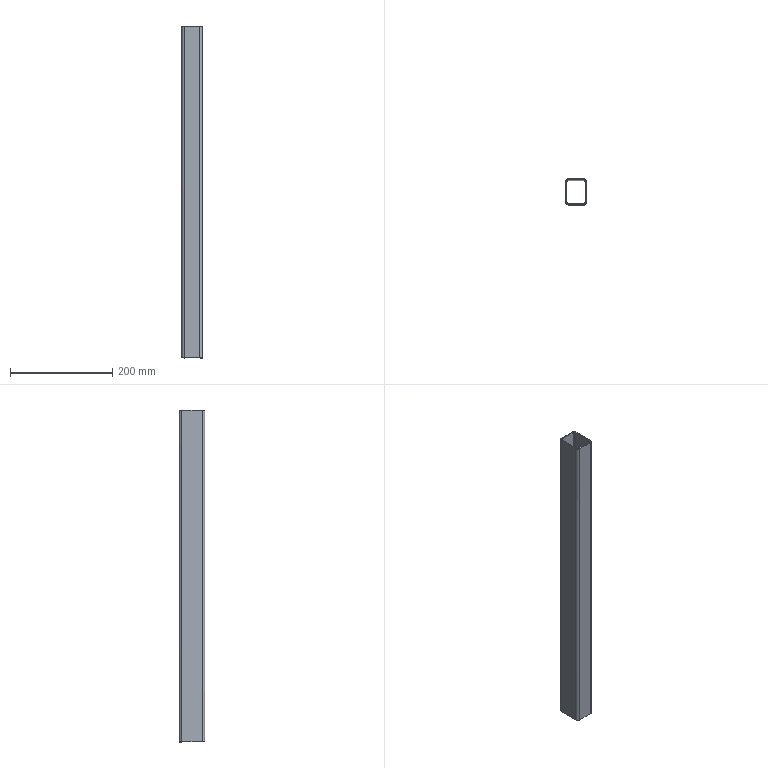Part | NX | features BREP 1 | 1 solid | 29 faces | box 40 x 50 x 649.59 mm | volume 214534 mm3 | plane 17 | cylinder 12 | commonest cylinder face diameters 6 x8 10 x4
STEP:
#1=CARTESIAN_POINT('',(2100.579,-584.17,553.344));
#2=VERTEX_POINT('',#1);
#3=CARTESIAN_POINT('',(2102.579,-584.17,553.344));
#4=VERTEX_POINT('',#3);
#5=CARTESIAN_POINT('',(2101.579,-584.17,553.344));
#6=DIRECTION('',(1.,0.,0.));
#7=VECTOR('',#6,1000.);
#8=LINE('',#5,#7);
#9=EDGE_CURVE('',#2,#4,#8,.T.);
#10=ORIENTED_EDGE('',*,*,#9,.T.);
#11=CARTESIAN_POINT('',(2102.579,-624.17,553.344));
#12=VERTEX_POINT('',#11);
#13=CARTESIAN_POINT('',(2102.579,-604.17,553.344));
#14=DIRECTION('',(0.,1.,0.));
#15=VECTOR('',#14,1000.);
#16=LINE('',#13,#15);
#17=EDGE_CURVE('',#12,#4,#16,.T.);
#18=ORIENTED_EDGE('',*,*,#17,.F.);
#19=CARTESIAN_POINT('',(2100.579,-624.17,553.344));
#20=VERTEX_POINT('',#19);
#21=CARTESIAN_POINT('',(2101.579,-624.17,553.344));
#22=DIRECTION('',(1.,0.,0.));
#23=VECTOR('',#22,1000.);
#24=LINE('',#21,#23);
#25=EDGE_CURVE('',#20,#12,#24,.T.);
#26=ORIENTED_EDGE('',*,*,#25,.F.);
#27=CARTESIAN_POINT('',(2100.579,-604.17,553.344));
#28=DIRECTION('',(0.,1.,0.));
#29=VECTOR('',#28,1000.);
#30=LINE('',#27,#29);
#31=EDGE_CURVE('',#20,#2,#30,.T.);
#32=ORIENTED_EDGE('',*,*,#31,.T.);
#33=EDGE_LOOP('',(#10,#18,#26,#32));
#34=FACE_BOUND('',#33,.T.);
#35=CARTESIAN_POINT('',(2102.579,-604.17,553.344));
#36=DIRECTION('',(0.,0.,1.));
#37=DIRECTION('',(1.,0.,0.));
#38=AXIS2_PLACEMENT_3D('',#35,#36,#37);
#39=PLANE('',#38);
#40=ADVANCED_FACE('',(#34),#39,.F.);
#41=CARTESIAN_POINT('',(2097.579,-581.17,553.344));
#42=VERTEX_POINT('',#41);
#43=CARTESIAN_POINT('',(2097.579,-579.17,553.344));
#44=VERTEX_POINT('',#43);
#45=CARTESIAN_POINT('',(2097.579,-580.17,553.344));
#46=DIRECTION('',(0.,1.,0.));
#47=VECTOR('',#46,1000.);
#48=LINE('',#45,#47);
#49=EDGE_CURVE('',#42,#44,#48,.T.);
#50=ORIENTED_EDGE('',*,*,#49,.T.);
#51=CARTESIAN_POINT('',(2097.579,-584.17,553.344));
#52=DIRECTION('',(0.,0.,1.));
#53=DIRECTION('',(1.,0.,0.));
#54=AXIS2_PLACEMENT_3D('',#51,#52,#53);
#55=CIRCLE('',#54,5.);
#56=EDGE_CURVE('',#4,#44,#55,.T.);
#57=ORIENTED_EDGE('',*,*,#56,.F.);
#58=ORIENTED_EDGE('',*,*,#9,.F.);
#59=CARTESIAN_POINT('',(2099.7,-582.049,553.344));
#60=VERTEX_POINT('',#59);
#61=CARTESIAN_POINT('',(2100.579,-584.17,553.344));
#62=CARTESIAN_POINT('',(2100.579,-583.383,553.344));
#63=CARTESIAN_POINT('',(2100.258,-582.606,553.344));
#64=CARTESIAN_POINT('',(2099.7,-582.049,553.344));
#65=B_SPLINE_CURVE_WITH_KNOTS('',3,(#61,#62,#63,#64),.UNSPECIFIED.,.F.,.F.,(4,4),(0.,1.),.UNSPECIFIED.);
#66=EDGE_CURVE('',#60,#2,#65,.F.);
#67=ORIENTED_EDGE('',*,*,#66,.F.);
#68=CARTESIAN_POINT('',(2099.7,-582.049,553.344));
#69=CARTESIAN_POINT('',(2099.143,-581.492,553.344));
#70=CARTESIAN_POINT('',(2098.367,-581.17,553.344));
#71=CARTESIAN_POINT('',(2097.579,-581.17,553.344));
#72=B_SPLINE_CURVE_WITH_KNOTS('',3,(#68,#69,#70,#71),.UNSPECIFIED.,.F.,.F.,(4,4),(0.,1.),.UNSPECIFIED.);
#73=EDGE_CURVE('',#42,#60,#72,.F.);
#74=ORIENTED_EDGE('',*,*,#73,.F.);
#75=EDGE_LOOP('',(#50,#57,#58,#67,#74));
#76=FACE_BOUND('',#75,.T.);
#77=CARTESIAN_POINT('',(2097.579,-579.17,553.344));
#78=DIRECTION('',(0.,0.,-1.));
#79=DIRECTION('',(0.9239,-0.3827,0.));
#80=AXIS2_PLACEMENT_3D('',#77,#78,#79);
#81=PLANE('',#80);
#82=ADVANCED_FACE('',(#76),#81,.T.);
#83=CARTESIAN_POINT('',(2099.7,-626.291,553.344));
#84=VERTEX_POINT('',#83);
#85=CARTESIAN_POINT('',(2097.579,-627.17,553.344));
#86=VERTEX_POINT('',#85);
#87=CARTESIAN_POINT('',(2097.579,-627.17,553.344));
#88=CARTESIAN_POINT('',(2098.366,-627.17,553.344));
#89=CARTESIAN_POINT('',(2099.142,-626.849,553.344));
#90=CARTESIAN_POINT('',(2099.7,-626.291,553.344));
#91=B_SPLINE_CURVE_WITH_KNOTS('',3,(#87,#88,#89,#90),.UNSPECIFIED.,.F.,.F.,(4,4),(0.,1.),.UNSPECIFIED.);
#92=EDGE_CURVE('',#84,#86,#91,.F.);
#93=ORIENTED_EDGE('',*,*,#92,.T.);
#94=CARTESIAN_POINT('',(2097.579,-627.17,1202.934));
#95=VERTEX_POINT('',#94);
#96=CARTESIAN_POINT('',(2097.579,-627.17,878.139));
#97=DIRECTION('',(0.,0.,1.));
#98=VECTOR('',#97,1000.);
#99=LINE('',#96,#98);
#100=EDGE_CURVE('',#86,#95,#99,.T.);
#101=ORIENTED_EDGE('',*,*,#100,.T.);
#102=CARTESIAN_POINT('',(2099.7,-626.291,1202.934));
#103=VERTEX_POINT('',#102);
#104=CARTESIAN_POINT('',(2097.579,-624.17,1202.934));
#105=DIRECTION('',(0.,0.,1.));
#106=DIRECTION('',(1.,0.,0.));
#107=AXIS2_PLACEMENT_3D('',#104,#105,#106);
#108=CIRCLE('',#107,3.);
#109=EDGE_CURVE('',#95,#103,#108,.T.);
#110=ORIENTED_EDGE('',*,*,#109,.T.);
#111=CARTESIAN_POINT('',(2099.7,-626.291,902.349));
#112=DIRECTION('',(0.,0.,1.));
#113=VECTOR('',#112,1000.);
#114=LINE('',#111,#113);
#115=EDGE_CURVE('',#84,#103,#114,.T.);
#116=ORIENTED_EDGE('',*,*,#115,.F.);
#117=EDGE_LOOP('',(#93,#101,#110,#116));
#118=FACE_BOUND('',#117,.T.);
#119=CARTESIAN_POINT('',(2097.579,-624.17,902.349));
#120=DIRECTION('',(0.,0.,1.));
#121=DIRECTION('',(-0.7071,0.7071,0.));
#122=AXIS2_PLACEMENT_3D('',#119,#120,#121);
#123=CYLINDRICAL_SURFACE('',#122,3.);
#124=ADVANCED_FACE('',(#118),#123,.F.);
#125=CARTESIAN_POINT('',(2100.579,-624.17,1202.934));
#126=VERTEX_POINT('',#125);
#127=CARTESIAN_POINT('',(2097.579,-624.17,1202.934));
#128=DIRECTION('',(0.,0.,1.));
#129=DIRECTION('',(1.,0.,0.));
#130=AXIS2_PLACEMENT_3D('',#127,#128,#129);
#131=CIRCLE('',#130,3.);
#132=EDGE_CURVE('',#103,#126,#131,.T.);
#133=ORIENTED_EDGE('',*,*,#132,.T.);
#134=CARTESIAN_POINT('',(2100.579,-624.17,878.139));
#135=DIRECTION('',(0.,0.,1.));
#136=VECTOR('',#135,1000.);
#137=LINE('',#134,#136);
#138=EDGE_CURVE('',#20,#126,#137,.T.);
#139=ORIENTED_EDGE('',*,*,#138,.F.);
#140=CARTESIAN_POINT('',(2099.7,-626.291,553.344));
#141=CARTESIAN_POINT('',(2100.257,-625.735,553.344));
#142=CARTESIAN_POINT('',(2100.579,-624.959,553.344));
#143=CARTESIAN_POINT('',(2100.579,-624.17,553.344));
#144=B_SPLINE_CURVE_WITH_KNOTS('',3,(#140,#141,#142,#143),.UNSPECIFIED.,.F.,.F.,(4,4),(0.,1.),.UNSPECIFIED.);
#145=EDGE_CURVE('',#20,#84,#144,.F.);
#146=ORIENTED_EDGE('',*,*,#145,.T.);
#147=ORIENTED_EDGE('',*,*,#115,.T.);
#148=EDGE_LOOP('',(#133,#139,#146,#147));
#149=FACE_BOUND('',#148,.T.);
#150=CARTESIAN_POINT('',(2097.579,-624.17,902.349));
#151=DIRECTION('',(0.,0.,1.));
#152=DIRECTION('',(0.7071,-0.7071,0.));
#153=AXIS2_PLACEMENT_3D('',#150,#151,#152);
#154=CYLINDRICAL_SURFACE('',#153,3.);
#155=ADVANCED_FACE('',(#149),#154,.F.);
#156=ORIENTED_EDGE('',*,*,#138,.T.);
#157=CARTESIAN_POINT('',(2100.579,-584.17,1202.934));
#158=VERTEX_POINT('',#157);
#159=CARTESIAN_POINT('',(2100.579,-604.17,1202.934));
#160=DIRECTION('',(0.,-1.,0.));
#161=VECTOR('',#160,1000.);
#162=LINE('',#159,#161);
#163=EDGE_CURVE('',#158,#126,#162,.T.);
#164=ORIENTED_EDGE('',*,*,#163,.F.);
#165=CARTESIAN_POINT('',(2100.579,-584.17,902.349));
#166=DIRECTION('',(0.,0.,1.));
#167=VECTOR('',#166,1000.);
#168=LINE('',#165,#167);
#169=EDGE_CURVE('',#2,#158,#168,.T.);
#170=ORIENTED_EDGE('',*,*,#169,.F.);
#171=ORIENTED_EDGE('',*,*,#31,.F.);
#172=EDGE_LOOP('',(#156,#164,#170,#171));
#173=FACE_BOUND('',#172,.T.);
#174=CARTESIAN_POINT('',(2100.579,-579.17,587.764));
#175=DIRECTION('',(-1.,0.,0.));
#176=DIRECTION('',(0.,-1.,0.));
#177=AXIS2_PLACEMENT_3D('',#174,#175,#176);
#178=PLANE('',#177);
#179=ADVANCED_FACE('',(#173),#178,.T.);
#180=ORIENTED_EDGE('',*,*,#66,.T.);
#181=ORIENTED_EDGE('',*,*,#169,.T.);
#182=CARTESIAN_POINT('',(2099.7,-582.049,1202.934));
#183=VERTEX_POINT('',#182);
#184=CARTESIAN_POINT('',(2097.579,-584.17,1202.934));
#185=DIRECTION('',(0.,0.,1.));
#186=DIRECTION('',(1.,0.,0.));
#187=AXIS2_PLACEMENT_3D('',#184,#185,#186);
#188=CIRCLE('',#187,3.);
#189=EDGE_CURVE('',#158,#183,#188,.T.);
#190=ORIENTED_EDGE('',*,*,#189,.T.);
#191=CARTESIAN_POINT('',(2099.7,-582.049,902.349));
#192=DIRECTION('',(0.,0.,1.));
#193=VECTOR('',#192,1000.);
#194=LINE('',#191,#193);
#195=EDGE_CURVE('',#60,#183,#194,.T.);
#196=ORIENTED_EDGE('',*,*,#195,.F.);
#197=EDGE_LOOP('',(#180,#181,#190,#196));
#198=FACE_BOUND('',#197,.T.);
#199=CARTESIAN_POINT('',(2097.579,-584.17,902.349));
#200=DIRECTION('',(0.,0.,1.));
#201=DIRECTION('',(-0.7071,-0.7071,0.));
#202=AXIS2_PLACEMENT_3D('',#199,#200,#201);
#203=CYLINDRICAL_SURFACE('',#202,3.);
#204=ADVANCED_FACE('',(#198),#203,.F.);
#205=CARTESIAN_POINT('',(2097.579,-581.17,1202.934));
#206=VERTEX_POINT('',#205);
#207=CARTESIAN_POINT('',(2097.579,-584.17,1202.934));
#208=DIRECTION('',(0.,0.,1.));
#209=DIRECTION('',(1.,0.,0.));
#210=AXIS2_PLACEMENT_3D('',#207,#208,#209);
#211=CIRCLE('',#210,3.);
#212=EDGE_CURVE('',#183,#206,#211,.T.);
#213=ORIENTED_EDGE('',*,*,#212,.T.);
#214=CARTESIAN_POINT('',(2097.579,-581.17,878.139));
#215=DIRECTION('',(0.,0.,1.));
#216=VECTOR('',#215,1000.);
#217=LINE('',#214,#216);
#218=EDGE_CURVE('',#42,#206,#217,.T.);
#219=ORIENTED_EDGE('',*,*,#218,.F.);
#220=ORIENTED_EDGE('',*,*,#73,.T.);
#221=ORIENTED_EDGE('',*,*,#195,.T.);
#222=EDGE_LOOP('',(#213,#219,#220,#221));
#223=FACE_BOUND('',#222,.T.);
#224=CARTESIAN_POINT('',(2097.579,-584.17,902.349));
#225=DIRECTION('',(0.,0.,1.));
#226=DIRECTION('',(0.7071,0.7071,0.));
#227=AXIS2_PLACEMENT_3D('',#224,#225,#226);
#228=CYLINDRICAL_SURFACE('',#227,3.);
#229=ADVANCED_FACE('',(#223),#228,.F.);
#230=CARTESIAN_POINT('',(2067.579,-581.17,553.344));
#231=VERTEX_POINT('',#230);
#232=CARTESIAN_POINT('',(2082.579,-581.17,553.344));
#233=DIRECTION('',(1.,0.,0.));
#234=VECTOR('',#233,1000.);
#235=LINE('',#232,#234);
#236=EDGE_CURVE('',#231,#42,#235,.T.);
#237=ORIENTED_EDGE('',*,*,#236,.T.);
#238=ORIENTED_EDGE('',*,*,#218,.T.);
#239=CARTESIAN_POINT('',(2067.579,-581.17,1202.934));
#240=VERTEX_POINT('',#239);
#241=CARTESIAN_POINT('',(2082.579,-581.17,1202.934));
#242=DIRECTION('',(-1.,0.,0.));
#243=VECTOR('',#242,1000.);
#244=LINE('',#241,#243);
#245=EDGE_CURVE('',#206,#240,#244,.T.);
#246=ORIENTED_EDGE('',*,*,#245,.T.);
#247=CARTESIAN_POINT('',(2067.579,-581.17,902.349));
#248=DIRECTION('',(0.,0.,1.));
#249=VECTOR('',#248,1000.);
#250=LINE('',#247,#249);
#251=EDGE_CURVE('',#231,#240,#250,.T.);
#252=ORIENTED_EDGE('',*,*,#251,.F.);
#253=EDGE_LOOP('',(#237,#238,#246,#252));
#254=FACE_BOUND('',#253,.T.);
#255=CARTESIAN_POINT('',(2102.579,-581.17,587.764));
#256=DIRECTION('',(0.,1.,0.));
#257=DIRECTION('',(-1.,0.,0.));
#258=AXIS2_PLACEMENT_3D('',#255,#256,#257);
#259=PLANE('',#258);
#260=ADVANCED_FACE('',(#254),#259,.F.);
#261=CARTESIAN_POINT('',(2067.579,-579.17,553.344));
#262=VERTEX_POINT('',#261);
#263=CARTESIAN_POINT('',(2067.579,-579.17,1202.934));
#264=VERTEX_POINT('',#263);
#265=CARTESIAN_POINT('',(2067.579,-579.17,902.349));
#266=DIRECTION('',(0.,0.,1.));
#267=VECTOR('',#266,1000.);
#268=LINE('',#265,#267);
#269=EDGE_CURVE('',#262,#264,#268,.T.);
#270=ORIENTED_EDGE('',*,*,#269,.T.);
#271=CARTESIAN_POINT('',(2097.579,-579.17,1202.934));
#272=VERTEX_POINT('',#271);
#273=CARTESIAN_POINT('',(2082.579,-579.17,1202.934));
#274=DIRECTION('',(-1.,0.,0.));
#275=VECTOR('',#274,1000.);
#276=LINE('',#273,#275);
#277=EDGE_CURVE('',#272,#264,#276,.T.);
#278=ORIENTED_EDGE('',*,*,#277,.F.);
#279=CARTESIAN_POINT('',(2097.579,-579.17,902.349));
#280=DIRECTION('',(0.,0.,1.));
#281=VECTOR('',#280,1000.);
#282=LINE('',#279,#281);
#283=EDGE_CURVE('',#44,#272,#282,.T.);
#284=ORIENTED_EDGE('',*,*,#283,.F.);
#285=CARTESIAN_POINT('',(2082.579,-579.17,553.344));
#286=DIRECTION('',(1.,0.,0.));
#287=VECTOR('',#286,1000.);
#288=LINE('',#285,#287);
#289=EDGE_CURVE('',#262,#44,#288,.T.);
#290=ORIENTED_EDGE('',*,*,#289,.F.);
#291=EDGE_LOOP('',(#270,#278,#284,#290));
#292=FACE_BOUND('',#291,.T.);
#293=CARTESIAN_POINT('',(2102.579,-579.17,587.764));
#294=DIRECTION('',(0.,1.,0.));
#295=DIRECTION('',(-1.,0.,0.));
#296=AXIS2_PLACEMENT_3D('',#293,#294,#295);
#297=PLANE('',#296);
#298=ADVANCED_FACE('',(#292),#297,.T.);
#299=ORIENTED_EDGE('',*,*,#283,.T.);
#300=CARTESIAN_POINT('',(2102.579,-584.17,1202.934));
#301=VERTEX_POINT('',#300);
#302=CARTESIAN_POINT('',(2097.579,-584.17,1202.934));
#303=DIRECTION('',(0.,0.,1.));
#304=DIRECTION('',(1.,0.,0.));
#305=AXIS2_PLACEMENT_3D('',#302,#303,#304);
#306=CIRCLE('',#305,5.);
#307=EDGE_CURVE('',#301,#272,#306,.T.);
#308=ORIENTED_EDGE('',*,*,#307,.F.);
#309=CARTESIAN_POINT('',(2102.579,-584.17,878.139));
#310=DIRECTION('',(0.,0.,1.));
#311=VECTOR('',#310,1000.);
#312=LINE('',#309,#311);
#313=EDGE_CURVE('',#4,#301,#312,.T.);
#314=ORIENTED_EDGE('',*,*,#313,.F.);
#315=ORIENTED_EDGE('',*,*,#56,.T.);
#316=EDGE_LOOP('',(#299,#308,#314,#315));
#317=FACE_BOUND('',#316,.T.);
#318=CARTESIAN_POINT('',(2097.579,-584.17,902.349));
#319=DIRECTION('',(0.,0.,1.));
#320=DIRECTION('',(1.,0.,0.));
#321=AXIS2_PLACEMENT_3D('',#318,#319,#320);
#322=CYLINDRICAL_SURFACE('',#321,5.);
#323=ADVANCED_FACE('',(#317),#322,.T.);
#324=ORIENTED_EDGE('',*,*,#17,.T.);
#325=ORIENTED_EDGE('',*,*,#313,.T.);
#326=CARTESIAN_POINT('',(2102.579,-624.17,1202.934));
#327=VERTEX_POINT('',#326);
#328=CARTESIAN_POINT('',(2102.579,-604.17,1202.934));
#329=DIRECTION('',(0.,-1.,0.));
#330=VECTOR('',#329,1000.);
#331=LINE('',#328,#330);
#332=EDGE_CURVE('',#301,#327,#331,.T.);
#333=ORIENTED_EDGE('',*,*,#332,.T.);
#334=CARTESIAN_POINT('',(2102.579,-624.17,902.349));
#335=DIRECTION('',(0.,0.,1.));
#336=VECTOR('',#335,1000.);
#337=LINE('',#334,#336);
#338=EDGE_CURVE('',#12,#327,#337,.T.);
#339=ORIENTED_EDGE('',*,*,#338,.F.);
#340=EDGE_LOOP('',(#324,#325,#333,#339));
#341=FACE_BOUND('',#340,.T.);
#342=CARTESIAN_POINT('',(2102.579,-579.17,587.764));
#343=DIRECTION('',(-1.,0.,0.));
#344=DIRECTION('',(0.,-1.,0.));
#345=AXIS2_PLACEMENT_3D('',#342,#343,#344);
#346=PLANE('',#345);
#347=ADVANCED_FACE('',(#341),#346,.F.);
#348=CARTESIAN_POINT('',(2097.579,-629.17,553.344));
#349=VERTEX_POINT('',#348);
#350=CARTESIAN_POINT('',(2097.579,-629.17,1202.934));
#351=VERTEX_POINT('',#350);
#352=CARTESIAN_POINT('',(2097.579,-629.17,878.139));
#353=DIRECTION('',(0.,0.,1.));
#354=VECTOR('',#353,1000.);
#355=LINE('',#352,#354);
#356=EDGE_CURVE('',#349,#351,#355,.T.);
#357=ORIENTED_EDGE('',*,*,#356,.F.);
#358=CARTESIAN_POINT('',(2102.579,-624.17,553.344));
#359=CARTESIAN_POINT('',(2102.579,-625.483,553.344));
#360=CARTESIAN_POINT('',(2101.492,-628.084,553.344));
#361=CARTESIAN_POINT('',(2098.894,-629.17,553.344));
#362=CARTESIAN_POINT('',(2097.579,-629.17,553.344));
#363=B_SPLINE_CURVE_WITH_KNOTS('',3,(#358,#359,#360,#361,#362),.UNSPECIFIED.,.F.,.F.,(4,1,4),(0.,0.5,1.),.UNSPECIFIED.);
#364=EDGE_CURVE('',#12,#349,#363,.T.);
#365=ORIENTED_EDGE('',*,*,#364,.F.);
#366=ORIENTED_EDGE('',*,*,#338,.T.);
#367=CARTESIAN_POINT('',(2097.579,-624.17,1202.934));
#368=DIRECTION('',(0.,0.,1.));
#369=DIRECTION('',(1.,0.,0.));
#370=AXIS2_PLACEMENT_3D('',#367,#368,#369);
#371=CIRCLE('',#370,5.);
#372=EDGE_CURVE('',#351,#327,#371,.T.);
#373=ORIENTED_EDGE('',*,*,#372,.F.);
#374=EDGE_LOOP('',(#357,#365,#366,#373));
#375=FACE_BOUND('',#374,.T.);
#376=CARTESIAN_POINT('',(2097.579,-624.17,902.349));
#377=DIRECTION('',(0.,0.,1.));
#378=DIRECTION('',(0.,-1.,0.));
#379=AXIS2_PLACEMENT_3D('',#376,#377,#378);
#380=CYLINDRICAL_SURFACE('',#379,5.);
#381=ADVANCED_FACE('',(#375),#380,.T.);
#382=ORIENTED_EDGE('',*,*,#364,.T.);
#383=CARTESIAN_POINT('',(2097.579,-628.17,553.344));
#384=DIRECTION('',(0.,1.,0.));
#385=VECTOR('',#384,1000.);
#386=LINE('',#383,#385);
#387=EDGE_CURVE('',#349,#86,#386,.T.);
#388=ORIENTED_EDGE('',*,*,#387,.T.);
#389=ORIENTED_EDGE('',*,*,#92,.F.);
#390=ORIENTED_EDGE('',*,*,#145,.F.);
#391=ORIENTED_EDGE('',*,*,#25,.T.);
#392=EDGE_LOOP('',(#382,#388,#389,#390,#391));
#393=FACE_BOUND('',#392,.T.);
#394=CARTESIAN_POINT('',(2102.579,-624.17,553.344));
#395=DIRECTION('',(0.,0.,-1.));
#396=DIRECTION('',(-0.3827,-0.9239,0.));
#397=AXIS2_PLACEMENT_3D('',#394,#395,#396);
#398=PLANE('',#397);
#399=ADVANCED_FACE('',(#393),#398,.T.);
#400=CARTESIAN_POINT('',(2067.579,-627.17,1202.934));
#401=VERTEX_POINT('',#400);
#402=CARTESIAN_POINT('',(2082.579,-627.17,1202.934));
#403=DIRECTION('',(1.,0.,0.));
#404=VECTOR('',#403,1000.);
#405=LINE('',#402,#404);
#406=EDGE_CURVE('',#401,#95,#405,.T.);
#407=ORIENTED_EDGE('',*,*,#406,.T.);
#408=ORIENTED_EDGE('',*,*,#100,.F.);
#409=CARTESIAN_POINT('',(2067.579,-627.17,553.344));
#410=VERTEX_POINT('',#409);
#411=CARTESIAN_POINT('',(2082.579,-627.17,553.344));
#412=DIRECTION('',(1.,0.,0.));
#413=VECTOR('',#412,1000.);
#414=LINE('',#411,#413);
#415=EDGE_CURVE('',#410,#86,#414,.T.);
#416=ORIENTED_EDGE('',*,*,#415,.F.);
#417=CARTESIAN_POINT('',(2067.579,-627.17,902.349));
#418=DIRECTION('',(0.,0.,1.));
#419=VECTOR('',#418,1000.);
#420=LINE('',#417,#419);
#421=EDGE_CURVE('',#410,#401,#420,.T.);
#422=ORIENTED_EDGE('',*,*,#421,.T.);
#423=EDGE_LOOP('',(#407,#408,#416,#422));
#424=FACE_BOUND('',#423,.T.);
#425=CARTESIAN_POINT('',(2062.579,-627.17,587.764));
#426=DIRECTION('',(0.,-1.,0.));
#427=DIRECTION('',(1.,0.,0.));
#428=AXIS2_PLACEMENT_3D('',#425,#426,#427);
#429=PLANE('',#428);
#430=ADVANCED_FACE('',(#424),#429,.F.);
#431=CARTESIAN_POINT('',(2067.579,-629.17,553.344));
#432=VERTEX_POINT('',#431);
#433=CARTESIAN_POINT('',(2067.579,-629.17,1202.934));
#434=VERTEX_POINT('',#433);
#435=CARTESIAN_POINT('',(2067.579,-629.17,902.349));
#436=DIRECTION('',(0.,0.,1.));
#437=VECTOR('',#436,1000.);
#438=LINE('',#435,#437);
#439=EDGE_CURVE('',#432,#434,#438,.T.);
#440=ORIENTED_EDGE('',*,*,#439,.F.);
#441=CARTESIAN_POINT('',(2082.579,-629.17,553.344));
#442=DIRECTION('',(1.,0.,0.));
#443=VECTOR('',#442,1000.);
#444=LINE('',#441,#443);
#445=EDGE_CURVE('',#432,#349,#444,.T.);
#446=ORIENTED_EDGE('',*,*,#445,.T.);
#447=ORIENTED_EDGE('',*,*,#356,.T.);
#448=CARTESIAN_POINT('',(2082.579,-629.17,1202.934));
#449=DIRECTION('',(1.,0.,0.));
#450=VECTOR('',#449,1000.);
#451=LINE('',#448,#450);
#452=EDGE_CURVE('',#434,#351,#451,.T.);
#453=ORIENTED_EDGE('',*,*,#452,.F.);
#454=EDGE_LOOP('',(#440,#446,#447,#453));
#455=FACE_BOUND('',#454,.T.);
#456=CARTESIAN_POINT('',(2062.579,-629.17,587.764));
#457=DIRECTION('',(0.,-1.,0.));
#458=DIRECTION('',(1.,0.,0.));
#459=AXIS2_PLACEMENT_3D('',#456,#457,#458);
#460=PLANE('',#459);
#461=ADVANCED_FACE('',(#455),#460,.T.);
#462=CARTESIAN_POINT('',(2065.457,-582.049,1202.934));
#463=VERTEX_POINT('',#462);
#464=CARTESIAN_POINT('',(2064.579,-584.17,1202.934));
#465=VERTEX_POINT('',#464);
#466=CARTESIAN_POINT('',(2067.579,-584.17,1202.934));
#467=DIRECTION('',(0.,0.,1.));
#468=DIRECTION('',(1.,0.,0.));
#469=AXIS2_PLACEMENT_3D('',#466,#467,#468);
#470=CIRCLE('',#469,3.);
#471=EDGE_CURVE('',#463,#465,#470,.T.);
#472=ORIENTED_EDGE('',*,*,#471,.T.);
#473=CARTESIAN_POINT('',(2064.579,-584.17,553.344));
#474=VERTEX_POINT('',#473);
#475=CARTESIAN_POINT('',(2064.579,-584.17,878.139));
#476=DIRECTION('',(0.,0.,1.));
#477=VECTOR('',#476,1000.);
#478=LINE('',#475,#477);
#479=EDGE_CURVE('',#474,#465,#478,.T.);
#480=ORIENTED_EDGE('',*,*,#479,.F.);
#481=CARTESIAN_POINT('',(2065.457,-582.049,553.344));
#482=VERTEX_POINT('',#481);
#483=CARTESIAN_POINT('',(2065.457,-582.049,553.344));
#484=CARTESIAN_POINT('',(2064.901,-582.605,553.344));
#485=CARTESIAN_POINT('',(2064.579,-583.381,553.344));
#486=CARTESIAN_POINT('',(2064.579,-584.17,553.344));
#487=B_SPLINE_CURVE_WITH_KNOTS('',3,(#483,#484,#485,#486),.UNSPECIFIED.,.F.,.F.,(4,4),(0.,1.),.UNSPECIFIED.);
#488=EDGE_CURVE('',#474,#482,#487,.F.);
#489=ORIENTED_EDGE('',*,*,#488,.T.);
#490=CARTESIAN_POINT('',(2065.457,-582.049,902.349));
#491=DIRECTION('',(0.,0.,1.));
#492=VECTOR('',#491,1000.);
#493=LINE('',#490,#492);
#494=EDGE_CURVE('',#482,#463,#493,.T.);
#495=ORIENTED_EDGE('',*,*,#494,.T.);
#496=EDGE_LOOP('',(#472,#480,#489,#495));
#497=FACE_BOUND('',#496,.T.);
#498=CARTESIAN_POINT('',(2067.579,-584.17,902.349));
#499=DIRECTION('',(0.,0.,1.));
#500=DIRECTION('',(-0.7071,0.7071,0.));
#501=AXIS2_PLACEMENT_3D('',#498,#499,#500);
#502=CYLINDRICAL_SURFACE('',#501,3.);
#503=ADVANCED_FACE('',(#497),#502,.F.);
#504=CARTESIAN_POINT('',(2067.579,-581.17,553.344));
#505=CARTESIAN_POINT('',(2066.791,-581.17,553.344));
#506=CARTESIAN_POINT('',(2066.015,-581.491,553.344));
#507=CARTESIAN_POINT('',(2065.457,-582.049,553.344));
#508=B_SPLINE_CURVE_WITH_KNOTS('',3,(#504,#505,#506,#507),.UNSPECIFIED.,.F.,.F.,(4,4),(0.,1.),.UNSPECIFIED.);
#509=EDGE_CURVE('',#482,#231,#508,.F.);
#510=ORIENTED_EDGE('',*,*,#509,.T.);
#511=ORIENTED_EDGE('',*,*,#251,.T.);
#512=CARTESIAN_POINT('',(2067.579,-584.17,1202.934));
#513=DIRECTION('',(0.,0.,1.));
#514=DIRECTION('',(1.,0.,0.));
#515=AXIS2_PLACEMENT_3D('',#512,#513,#514);
#516=CIRCLE('',#515,3.);
#517=EDGE_CURVE('',#240,#463,#516,.T.);
#518=ORIENTED_EDGE('',*,*,#517,.T.);
#519=ORIENTED_EDGE('',*,*,#494,.F.);
#520=EDGE_LOOP('',(#510,#511,#518,#519));
#521=FACE_BOUND('',#520,.T.);
#522=CARTESIAN_POINT('',(2067.579,-584.17,902.349));
#523=DIRECTION('',(0.,0.,1.));
#524=DIRECTION('',(0.7071,-0.7071,0.));
#525=AXIS2_PLACEMENT_3D('',#522,#523,#524);
#526=CYLINDRICAL_SURFACE('',#525,3.);
#527=ADVANCED_FACE('',(#521),#526,.F.);
#528=ORIENTED_EDGE('',*,*,#236,.F.);
#529=CARTESIAN_POINT('',(2067.579,-580.17,553.344));
#530=DIRECTION('',(0.,1.,0.));
#531=VECTOR('',#530,1000.);
#532=LINE('',#529,#531);
#533=EDGE_CURVE('',#231,#262,#532,.T.);
#534=ORIENTED_EDGE('',*,*,#533,.T.);
#535=ORIENTED_EDGE('',*,*,#289,.T.);
#536=ORIENTED_EDGE('',*,*,#49,.F.);
#537=EDGE_LOOP('',(#528,#534,#535,#536));
#538=FACE_BOUND('',#537,.T.);
#539=CARTESIAN_POINT('',(2082.579,-579.17,553.344));
#540=DIRECTION('',(0.,0.,1.));
#541=DIRECTION('',(1.,0.,0.));
#542=AXIS2_PLACEMENT_3D('',#539,#540,#541);
#543=PLANE('',#542);
#544=ADVANCED_FACE('',(#538),#543,.F.);
#545=CARTESIAN_POINT('',(2062.579,-584.17,553.344));
#546=VERTEX_POINT('',#545);
#547=CARTESIAN_POINT('',(2062.579,-584.17,1202.934));
#548=VERTEX_POINT('',#547);
#549=CARTESIAN_POINT('',(2062.579,-584.17,878.139));
#550=DIRECTION('',(0.,0.,1.));
#551=VECTOR('',#550,1000.);
#552=LINE('',#549,#551);
#553=EDGE_CURVE('',#546,#548,#552,.T.);
#554=ORIENTED_EDGE('',*,*,#553,.T.);
#555=CARTESIAN_POINT('',(2067.579,-584.17,1202.934));
#556=DIRECTION('',(0.,0.,1.));
#557=DIRECTION('',(1.,0.,0.));
#558=AXIS2_PLACEMENT_3D('',#555,#556,#557);
#559=CIRCLE('',#558,5.);
#560=EDGE_CURVE('',#264,#548,#559,.T.);
#561=ORIENTED_EDGE('',*,*,#560,.F.);
#562=ORIENTED_EDGE('',*,*,#269,.F.);
#563=CARTESIAN_POINT('',(2062.579,-584.17,553.344));
#564=CARTESIAN_POINT('',(2062.579,-582.857,553.344));
#565=CARTESIAN_POINT('',(2063.665,-580.256,553.344));
#566=CARTESIAN_POINT('',(2066.264,-579.17,553.344));
#567=CARTESIAN_POINT('',(2067.579,-579.17,553.344));
#568=B_SPLINE_CURVE_WITH_KNOTS('',3,(#563,#564,#565,#566,#567),.UNSPECIFIED.,.F.,.F.,(4,1,4),(0.,0.5,1.),.UNSPECIFIED.);
#569=EDGE_CURVE('',#546,#262,#568,.T.);
#570=ORIENTED_EDGE('',*,*,#569,.F.);
#571=EDGE_LOOP('',(#554,#561,#562,#570));
#572=FACE_BOUND('',#571,.T.);
#573=CARTESIAN_POINT('',(2067.579,-584.17,902.349));
#574=DIRECTION('',(0.,0.,1.));
#575=DIRECTION('',(0.,1.,0.));
#576=AXIS2_PLACEMENT_3D('',#573,#574,#575);
#577=CYLINDRICAL_SURFACE('',#576,5.);
#578=ADVANCED_FACE('',(#572),#577,.T.);
#579=ORIENTED_EDGE('',*,*,#471,.F.);
#580=ORIENTED_EDGE('',*,*,#517,.F.);
#581=ORIENTED_EDGE('',*,*,#245,.F.);
#582=ORIENTED_EDGE('',*,*,#212,.F.);
#583=ORIENTED_EDGE('',*,*,#189,.F.);
#584=ORIENTED_EDGE('',*,*,#163,.T.);
#585=ORIENTED_EDGE('',*,*,#132,.F.);
#586=ORIENTED_EDGE('',*,*,#109,.F.);
#587=ORIENTED_EDGE('',*,*,#406,.F.);
#588=CARTESIAN_POINT('',(2065.457,-626.291,1202.934));
#589=VERTEX_POINT('',#588);
#590=CARTESIAN_POINT('',(2067.579,-627.17,1202.934));
#591=CARTESIAN_POINT('',(2066.792,-627.17,1202.934));
#592=CARTESIAN_POINT('',(2066.015,-626.849,1202.934));
#593=CARTESIAN_POINT('',(2065.457,-626.291,1202.934));
#594=B_SPLINE_CURVE_WITH_KNOTS('',3,(#590,#591,#592,#593),.UNSPECIFIED.,.F.,.F.,(4,4),(0.,1.),.UNSPECIFIED.);
#595=EDGE_CURVE('',#589,#401,#594,.F.);
#596=ORIENTED_EDGE('',*,*,#595,.F.);
#597=CARTESIAN_POINT('',(2064.579,-624.17,1202.934));
#598=VERTEX_POINT('',#597);
#599=CARTESIAN_POINT('',(2065.457,-626.291,1202.934));
#600=CARTESIAN_POINT('',(2064.901,-625.735,1202.934));
#601=CARTESIAN_POINT('',(2064.579,-624.959,1202.934));
#602=CARTESIAN_POINT('',(2064.579,-624.17,1202.934));
#603=B_SPLINE_CURVE_WITH_KNOTS('',3,(#599,#600,#601,#602),.UNSPECIFIED.,.F.,.F.,(4,4),(0.,1.),.UNSPECIFIED.);
#604=EDGE_CURVE('',#598,#589,#603,.F.);
#605=ORIENTED_EDGE('',*,*,#604,.F.);
#606=CARTESIAN_POINT('',(2064.579,-604.17,1202.934));
#607=DIRECTION('',(0.,1.,0.));
#608=VECTOR('',#607,1000.);
#609=LINE('',#606,#608);
#610=EDGE_CURVE('',#598,#465,#609,.T.);
#611=ORIENTED_EDGE('',*,*,#610,.T.);
#612=EDGE_LOOP('',(#579,#580,#581,#582,#583,#584,#585,#586,#587,#596,#605,#611));
#613=FACE_BOUND('',#612,.T.);
#614=CARTESIAN_POINT('',(2062.579,-624.17,1202.934));
#615=VERTEX_POINT('',#614);
#616=CARTESIAN_POINT('',(2062.579,-604.17,1202.934));
#617=DIRECTION('',(0.,1.,0.));
#618=VECTOR('',#617,1000.);
#619=LINE('',#616,#618);
#620=EDGE_CURVE('',#615,#548,#619,.T.);
#621=ORIENTED_EDGE('',*,*,#620,.F.);
#622=CARTESIAN_POINT('',(2067.579,-624.17,1202.934));
#623=DIRECTION('',(0.,0.,1.));
#624=DIRECTION('',(1.,0.,0.));
#625=AXIS2_PLACEMENT_3D('',#622,#623,#624);
#626=CIRCLE('',#625,5.);
#627=EDGE_CURVE('',#615,#434,#626,.T.);
#628=ORIENTED_EDGE('',*,*,#627,.T.);
#629=ORIENTED_EDGE('',*,*,#452,.T.);
#630=ORIENTED_EDGE('',*,*,#372,.T.);
#631=ORIENTED_EDGE('',*,*,#332,.F.);
#632=ORIENTED_EDGE('',*,*,#307,.T.);
#633=ORIENTED_EDGE('',*,*,#277,.T.);
#634=ORIENTED_EDGE('',*,*,#560,.T.);
#635=EDGE_LOOP('',(#621,#628,#629,#630,#631,#632,#633,#634));
#636=FACE_BOUND('',#635,.T.);
#637=CARTESIAN_POINT('',(2082.579,-314.585,1202.934));
#638=DIRECTION('',(0.,0.,1.));
#639=DIRECTION('',(-1.,0.,0.));
#640=AXIS2_PLACEMENT_3D('',#637,#638,#639);
#641=PLANE('',#640);
#642=ADVANCED_FACE('',(#613,#636),#641,.T.);
#643=ORIENTED_EDGE('',*,*,#445,.F.);
#644=CARTESIAN_POINT('',(2067.579,-628.17,553.344));
#645=DIRECTION('',(0.,-1.,0.));
#646=VECTOR('',#645,1000.);
#647=LINE('',#644,#646);
#648=EDGE_CURVE('',#410,#432,#647,.T.);
#649=ORIENTED_EDGE('',*,*,#648,.F.);
#650=ORIENTED_EDGE('',*,*,#415,.T.);
#651=ORIENTED_EDGE('',*,*,#387,.F.);
#652=EDGE_LOOP('',(#643,#649,#650,#651));
#653=FACE_BOUND('',#652,.T.);
#654=CARTESIAN_POINT('',(2082.579,-629.17,553.344));
#655=DIRECTION('',(0.,0.,1.));
#656=DIRECTION('',(1.,0.,0.));
#657=AXIS2_PLACEMENT_3D('',#654,#655,#656);
#658=PLANE('',#657);
#659=ADVANCED_FACE('',(#653),#658,.F.);
#660=ORIENTED_EDGE('',*,*,#595,.T.);
#661=ORIENTED_EDGE('',*,*,#421,.F.);
#662=CARTESIAN_POINT('',(2065.457,-626.291,553.344));
#663=VERTEX_POINT('',#662);
#664=CARTESIAN_POINT('',(2065.457,-626.291,553.344));
#665=CARTESIAN_POINT('',(2066.014,-626.848,553.344));
#666=CARTESIAN_POINT('',(2066.79,-627.17,553.344));
#667=CARTESIAN_POINT('',(2067.579,-627.17,553.344));
#668=B_SPLINE_CURVE_WITH_KNOTS('',3,(#664,#665,#666,#667),.UNSPECIFIED.,.F.,.F.,(4,4),(0.,1.),.UNSPECIFIED.);
#669=EDGE_CURVE('',#410,#663,#668,.F.);
#670=ORIENTED_EDGE('',*,*,#669,.T.);
#671=CARTESIAN_POINT('',(2065.457,-626.291,902.349));
#672=DIRECTION('',(0.,0.,1.));
#673=VECTOR('',#672,1000.);
#674=LINE('',#671,#673);
#675=EDGE_CURVE('',#663,#589,#674,.T.);
#676=ORIENTED_EDGE('',*,*,#675,.T.);
#677=EDGE_LOOP('',(#660,#661,#670,#676));
#678=FACE_BOUND('',#677,.T.);
#679=CARTESIAN_POINT('',(2067.579,-624.17,902.349));
#680=DIRECTION('',(0.,0.,1.));
#681=DIRECTION('',(-0.7071,-0.7071,0.));
#682=AXIS2_PLACEMENT_3D('',#679,#680,#681);
#683=CYLINDRICAL_SURFACE('',#682,3.);
#684=ADVANCED_FACE('',(#678),#683,.F.);
#685=CARTESIAN_POINT('',(2064.579,-624.17,553.344));
#686=VERTEX_POINT('',#685);
#687=CARTESIAN_POINT('',(2064.579,-624.17,553.344));
#688=CARTESIAN_POINT('',(2064.579,-624.958,553.344));
#689=CARTESIAN_POINT('',(2064.9,-625.733,553.344));
#690=CARTESIAN_POINT('',(2065.457,-626.291,553.344));
#691=B_SPLINE_CURVE_WITH_KNOTS('',3,(#687,#688,#689,#690),.UNSPECIFIED.,.F.,.F.,(4,4),(0.,1.),.UNSPECIFIED.);
#692=EDGE_CURVE('',#663,#686,#691,.F.);
#693=ORIENTED_EDGE('',*,*,#692,.T.);
#694=CARTESIAN_POINT('',(2064.579,-624.17,878.139));
#695=DIRECTION('',(0.,0.,1.));
#696=VECTOR('',#695,1000.);
#697=LINE('',#694,#696);
#698=EDGE_CURVE('',#686,#598,#697,.T.);
#699=ORIENTED_EDGE('',*,*,#698,.T.);
#700=ORIENTED_EDGE('',*,*,#604,.T.);
#701=ORIENTED_EDGE('',*,*,#675,.F.);
#702=EDGE_LOOP('',(#693,#699,#700,#701));
#703=FACE_BOUND('',#702,.T.);
#704=CARTESIAN_POINT('',(2067.579,-624.17,902.349));
#705=DIRECTION('',(0.,0.,1.));
#706=DIRECTION('',(0.7071,0.7071,0.));
#707=AXIS2_PLACEMENT_3D('',#704,#705,#706);
#708=CYLINDRICAL_SURFACE('',#707,3.);
#709=ADVANCED_FACE('',(#703),#708,.F.);
#710=CARTESIAN_POINT('',(2062.579,-624.17,553.344));
#711=VERTEX_POINT('',#710);
#712=CARTESIAN_POINT('',(2062.579,-624.17,878.139));
#713=DIRECTION('',(0.,0.,1.));
#714=VECTOR('',#713,1000.);
#715=LINE('',#712,#714);
#716=EDGE_CURVE('',#711,#615,#715,.T.);
#717=ORIENTED_EDGE('',*,*,#716,.F.);
#718=CARTESIAN_POINT('',(2067.579,-629.17,553.344));
#719=CARTESIAN_POINT('',(2066.265,-629.17,553.344));
#720=CARTESIAN_POINT('',(2063.665,-628.083,553.344));
#721=CARTESIAN_POINT('',(2062.579,-625.485,553.344));
#722=CARTESIAN_POINT('',(2062.579,-624.17,553.344));
#723=B_SPLINE_CURVE_WITH_KNOTS('',3,(#718,#719,#720,#721,#722),.UNSPECIFIED.,.F.,.F.,(4,1,4),(0.,0.5,1.),.UNSPECIFIED.);
#724=EDGE_CURVE('',#432,#711,#723,.T.);
#725=ORIENTED_EDGE('',*,*,#724,.F.);
#726=ORIENTED_EDGE('',*,*,#439,.T.);
#727=ORIENTED_EDGE('',*,*,#627,.F.);
#728=EDGE_LOOP('',(#717,#725,#726,#727));
#729=FACE_BOUND('',#728,.T.);
#730=CARTESIAN_POINT('',(2067.579,-624.17,902.349));
#731=DIRECTION('',(0.,0.,1.));
#732=DIRECTION('',(-1.,0.,0.));
#733=AXIS2_PLACEMENT_3D('',#730,#731,#732);
#734=CYLINDRICAL_SURFACE('',#733,5.);
#735=ADVANCED_FACE('',(#729),#734,.T.);
#736=ORIENTED_EDGE('',*,*,#698,.F.);
#737=CARTESIAN_POINT('',(2064.579,-604.17,553.344));
#738=DIRECTION('',(0.,1.,0.));
#739=VECTOR('',#738,1000.);
#740=LINE('',#737,#739);
#741=EDGE_CURVE('',#686,#474,#740,.T.);
#742=ORIENTED_EDGE('',*,*,#741,.T.);
#743=ORIENTED_EDGE('',*,*,#479,.T.);
#744=ORIENTED_EDGE('',*,*,#610,.F.);
#745=EDGE_LOOP('',(#736,#742,#743,#744));
#746=FACE_BOUND('',#745,.T.);
#747=CARTESIAN_POINT('',(2064.579,-629.17,587.764));
#748=DIRECTION('',(1.,0.,0.));
#749=DIRECTION('',(0.,1.,0.));
#750=AXIS2_PLACEMENT_3D('',#747,#748,#749);
#751=PLANE('',#750);
#752=ADVANCED_FACE('',(#746),#751,.T.);
#753=ORIENTED_EDGE('',*,*,#533,.F.);
#754=ORIENTED_EDGE('',*,*,#509,.F.);
#755=ORIENTED_EDGE('',*,*,#488,.F.);
#756=CARTESIAN_POINT('',(2063.579,-584.17,553.344));
#757=DIRECTION('',(1.,0.,0.));
#758=VECTOR('',#757,1000.);
#759=LINE('',#756,#758);
#760=EDGE_CURVE('',#546,#474,#759,.T.);
#761=ORIENTED_EDGE('',*,*,#760,.F.);
#762=ORIENTED_EDGE('',*,*,#569,.T.);
#763=EDGE_LOOP('',(#753,#754,#755,#761,#762));
#764=FACE_BOUND('',#763,.T.);
#765=CARTESIAN_POINT('',(2062.579,-584.17,553.344));
#766=DIRECTION('',(0.,0.,-1.));
#767=DIRECTION('',(0.3827,0.9239,0.));
#768=AXIS2_PLACEMENT_3D('',#765,#766,#767);
#769=PLANE('',#768);
#770=ADVANCED_FACE('',(#764),#769,.T.);
#771=CARTESIAN_POINT('',(2062.579,-604.17,553.344));
#772=DIRECTION('',(0.,1.,0.));
#773=VECTOR('',#772,1000.);
#774=LINE('',#771,#773);
#775=EDGE_CURVE('',#711,#546,#774,.T.);
#776=ORIENTED_EDGE('',*,*,#775,.F.);
#777=ORIENTED_EDGE('',*,*,#716,.T.);
#778=ORIENTED_EDGE('',*,*,#620,.T.);
#779=ORIENTED_EDGE('',*,*,#553,.F.);
#780=EDGE_LOOP('',(#776,#777,#778,#779));
#781=FACE_BOUND('',#780,.T.);
#782=CARTESIAN_POINT('',(2062.579,-629.17,587.764));
#783=DIRECTION('',(1.,0.,0.));
#784=DIRECTION('',(0.,1.,0.));
#785=AXIS2_PLACEMENT_3D('',#782,#783,#784);
#786=PLANE('',#785);
#787=ADVANCED_FACE('',(#781),#786,.F.);
#788=ORIENTED_EDGE('',*,*,#724,.T.);
#789=CARTESIAN_POINT('',(2063.579,-624.17,553.344));
#790=DIRECTION('',(1.,0.,0.));
#791=VECTOR('',#790,1000.);
#792=LINE('',#789,#791);
#793=EDGE_CURVE('',#711,#686,#792,.T.);
#794=ORIENTED_EDGE('',*,*,#793,.T.);
#795=ORIENTED_EDGE('',*,*,#692,.F.);
#796=ORIENTED_EDGE('',*,*,#669,.F.);
#797=ORIENTED_EDGE('',*,*,#648,.T.);
#798=EDGE_LOOP('',(#788,#794,#795,#796,#797));
#799=FACE_BOUND('',#798,.T.);
#800=CARTESIAN_POINT('',(2067.579,-629.17,553.344));
#801=DIRECTION('',(0.,0.,-1.));
#802=DIRECTION('',(-0.9239,0.3827,0.));
#803=AXIS2_PLACEMENT_3D('',#800,#801,#802);
#804=PLANE('',#803);
#805=ADVANCED_FACE('',(#799),#804,.T.);
#806=ORIENTED_EDGE('',*,*,#793,.F.);
#807=ORIENTED_EDGE('',*,*,#775,.T.);
#808=ORIENTED_EDGE('',*,*,#760,.T.);
#809=ORIENTED_EDGE('',*,*,#741,.F.);
#810=EDGE_LOOP('',(#806,#807,#808,#809));
#811=FACE_BOUND('',#810,.T.);
#812=CARTESIAN_POINT('',(2062.579,-604.17,553.344));
#813=DIRECTION('',(0.,0.,1.));
#814=DIRECTION('',(1.,0.,0.));
#815=AXIS2_PLACEMENT_3D('',#812,#813,#814);
#816=PLANE('',#815);
#817=ADVANCED_FACE('',(#811),#816,.F.);
#818=CLOSED_SHELL('',(#40,#82,#124,#155,#179,#204,#229,#260,#298,#323,#347,#381,#399,#430,#461,#503,#527,#544,#578,#642,#659,#684,#709,#735,#752,#770,#787,#805,#817));
#819=MANIFOLD_SOLID_BREP('',#818);
#820=(LENGTH_UNIT()NAMED_UNIT(*)SI_UNIT(.MILLI.,.METRE.));
#821=UNCERTAINTY_MEASURE_WITH_UNIT(LENGTH_MEASURE(0.0508),#820,'','');
#822=(NAMED_UNIT(*)PLANE_ANGLE_UNIT()SI_UNIT($,.RADIAN.));
#823=(NAMED_UNIT(*)SI_UNIT($,.STERADIAN.)SOLID_ANGLE_UNIT());
#824=(GEOMETRIC_REPRESENTATION_CONTEXT(3)GLOBAL_UNCERTAINTY_ASSIGNED_CONTEXT((#821))GLOBAL_UNIT_ASSIGNED_CONTEXT((#820,#822,#823))REPRESENTATION_CONTEXT('',''));
#825=ADVANCED_BREP_SHAPE_REPRESENTATION('',(#819),#824);